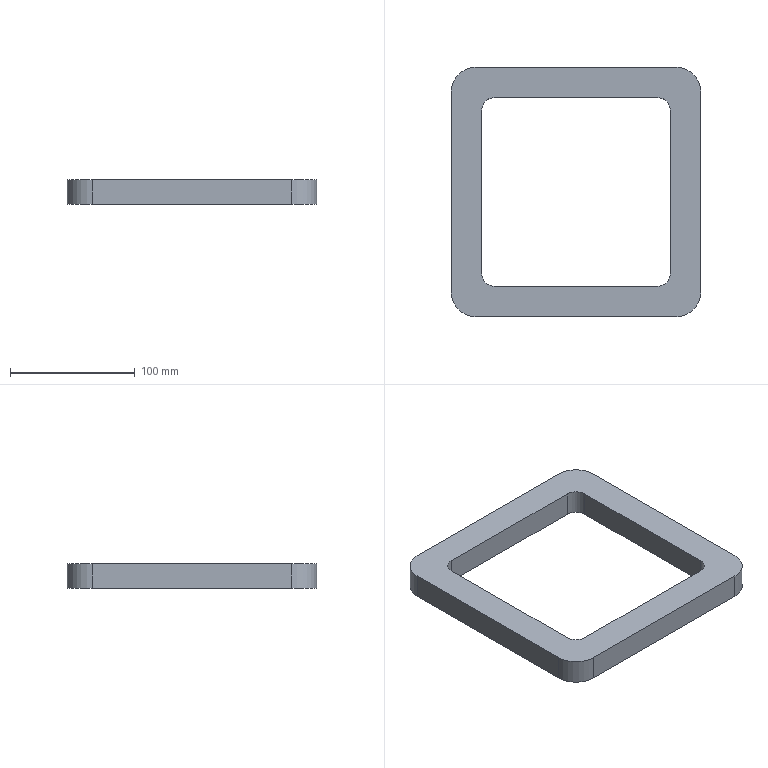Part | SolidWorks | features Fillet 2, Extrusion 1 | 1 solid | 18 faces | box 200 x 200 x 20 mm | volume 338830 mm3 | plane 10 | cylinder 8 | commonest cylinder face diameters 20 x4 40 x4
STEP:
#1=CARTESIAN_POINT('',(0.,180.,20.));
#2=VERTEX_POINT('',#1);
#3=CARTESIAN_POINT('',(0.,20.,20.));
#4=VERTEX_POINT('',#3);
#5=CARTESIAN_POINT('',(0.,0.,20.));
#6=DIRECTION('',(0.,-1.,0.));
#7=VECTOR('',#6,1000.);
#8=LINE('',#5,#7);
#9=EDGE_CURVE('',#2,#4,#8,.T.);
#10=ORIENTED_EDGE('',*,*,#9,.T.);
#11=CARTESIAN_POINT('',(20.,0.,20.));
#12=VERTEX_POINT('',#11);
#13=CARTESIAN_POINT('',(20.,20.,20.));
#14=DIRECTION('',(0.,0.,1.));
#15=DIRECTION('',(-1.,0.,0.));
#16=AXIS2_PLACEMENT_3D('',#13,#14,#15);
#17=CIRCLE('',#16,20.);
#18=EDGE_CURVE('',#4,#12,#17,.T.);
#19=ORIENTED_EDGE('',*,*,#18,.T.);
#20=CARTESIAN_POINT('',(180.,0.,20.));
#21=VERTEX_POINT('',#20);
#22=CARTESIAN_POINT('',(0.,0.,20.));
#23=DIRECTION('',(1.,0.,0.));
#24=VECTOR('',#23,1000.);
#25=LINE('',#22,#24);
#26=EDGE_CURVE('',#12,#21,#25,.T.);
#27=ORIENTED_EDGE('',*,*,#26,.T.);
#28=CARTESIAN_POINT('',(200.,20.,20.));
#29=VERTEX_POINT('',#28);
#30=CARTESIAN_POINT('',(180.,20.,20.));
#31=DIRECTION('',(0.,0.,1.));
#32=DIRECTION('',(-1.,0.,0.));
#33=AXIS2_PLACEMENT_3D('',#30,#31,#32);
#34=CIRCLE('',#33,20.);
#35=EDGE_CURVE('',#21,#29,#34,.T.);
#36=ORIENTED_EDGE('',*,*,#35,.T.);
#37=CARTESIAN_POINT('',(200.,180.,20.));
#38=VERTEX_POINT('',#37);
#39=CARTESIAN_POINT('',(200.,0.,20.));
#40=DIRECTION('',(0.,1.,0.));
#41=VECTOR('',#40,1000.);
#42=LINE('',#39,#41);
#43=EDGE_CURVE('',#29,#38,#42,.T.);
#44=ORIENTED_EDGE('',*,*,#43,.T.);
#45=CARTESIAN_POINT('',(180.,200.,20.));
#46=VERTEX_POINT('',#45);
#47=CARTESIAN_POINT('',(180.,180.,20.));
#48=DIRECTION('',(0.,0.,1.));
#49=DIRECTION('',(-1.,0.,0.));
#50=AXIS2_PLACEMENT_3D('',#47,#48,#49);
#51=CIRCLE('',#50,20.);
#52=EDGE_CURVE('',#38,#46,#51,.T.);
#53=ORIENTED_EDGE('',*,*,#52,.T.);
#54=CARTESIAN_POINT('',(20.,200.,20.));
#55=VERTEX_POINT('',#54);
#56=CARTESIAN_POINT('',(0.,200.,20.));
#57=DIRECTION('',(-1.,0.,0.));
#58=VECTOR('',#57,1000.);
#59=LINE('',#56,#58);
#60=EDGE_CURVE('',#46,#55,#59,.T.);
#61=ORIENTED_EDGE('',*,*,#60,.T.);
#62=CARTESIAN_POINT('',(20.,180.,20.));
#63=DIRECTION('',(0.,0.,1.));
#64=DIRECTION('',(-1.,0.,0.));
#65=AXIS2_PLACEMENT_3D('',#62,#63,#64);
#66=CIRCLE('',#65,20.);
#67=EDGE_CURVE('',#55,#2,#66,.T.);
#68=ORIENTED_EDGE('',*,*,#67,.T.);
#69=EDGE_LOOP('',(#10,#19,#27,#36,#44,#53,#61,#68));
#70=FACE_OUTER_BOUND('',#69,.T.);
#71=CARTESIAN_POINT('',(24.5,165.5,20.));
#72=VERTEX_POINT('',#71);
#73=CARTESIAN_POINT('',(24.5,34.5,20.));
#74=VERTEX_POINT('',#73);
#75=CARTESIAN_POINT('',(24.5,175.5,20.));
#76=DIRECTION('',(0.,-1.,0.));
#77=VECTOR('',#76,1000.);
#78=LINE('',#75,#77);
#79=EDGE_CURVE('',#72,#74,#78,.T.);
#80=ORIENTED_EDGE('',*,*,#79,.F.);
#81=CARTESIAN_POINT('',(34.5,175.5,20.));
#82=VERTEX_POINT('',#81);
#83=CARTESIAN_POINT('',(34.5,165.5,20.));
#84=DIRECTION('',(0.,0.,-1.));
#85=DIRECTION('',(-1.,0.,0.));
#86=AXIS2_PLACEMENT_3D('',#83,#84,#85);
#87=CIRCLE('',#86,10.);
#88=EDGE_CURVE('',#72,#82,#87,.T.);
#89=ORIENTED_EDGE('',*,*,#88,.T.);
#90=CARTESIAN_POINT('',(165.5,175.5,20.));
#91=VERTEX_POINT('',#90);
#92=CARTESIAN_POINT('',(24.5,175.5,20.));
#93=DIRECTION('',(-1.,0.,0.));
#94=VECTOR('',#93,1000.);
#95=LINE('',#92,#94);
#96=EDGE_CURVE('',#91,#82,#95,.T.);
#97=ORIENTED_EDGE('',*,*,#96,.F.);
#98=CARTESIAN_POINT('',(175.5,165.5,20.));
#99=VERTEX_POINT('',#98);
#100=CARTESIAN_POINT('',(165.5,165.5,20.));
#101=DIRECTION('',(0.,0.,-1.));
#102=DIRECTION('',(-1.,0.,0.));
#103=AXIS2_PLACEMENT_3D('',#100,#101,#102);
#104=CIRCLE('',#103,10.);
#105=EDGE_CURVE('',#91,#99,#104,.T.);
#106=ORIENTED_EDGE('',*,*,#105,.T.);
#107=CARTESIAN_POINT('',(175.5,34.5,20.));
#108=VERTEX_POINT('',#107);
#109=CARTESIAN_POINT('',(175.5,175.5,20.));
#110=DIRECTION('',(0.,1.,0.));
#111=VECTOR('',#110,1000.);
#112=LINE('',#109,#111);
#113=EDGE_CURVE('',#108,#99,#112,.T.);
#114=ORIENTED_EDGE('',*,*,#113,.F.);
#115=CARTESIAN_POINT('',(165.5,24.5,20.));
#116=VERTEX_POINT('',#115);
#117=CARTESIAN_POINT('',(165.5,34.5,20.));
#118=DIRECTION('',(0.,0.,-1.));
#119=DIRECTION('',(-1.,0.,0.));
#120=AXIS2_PLACEMENT_3D('',#117,#118,#119);
#121=CIRCLE('',#120,10.);
#122=EDGE_CURVE('',#108,#116,#121,.T.);
#123=ORIENTED_EDGE('',*,*,#122,.T.);
#124=CARTESIAN_POINT('',(34.5,24.5,20.));
#125=VERTEX_POINT('',#124);
#126=CARTESIAN_POINT('',(24.5,24.5,20.));
#127=DIRECTION('',(1.,0.,0.));
#128=VECTOR('',#127,1000.);
#129=LINE('',#126,#128);
#130=EDGE_CURVE('',#125,#116,#129,.T.);
#131=ORIENTED_EDGE('',*,*,#130,.F.);
#132=CARTESIAN_POINT('',(34.5,34.5,20.));
#133=DIRECTION('',(0.,0.,-1.));
#134=DIRECTION('',(-1.,0.,0.));
#135=AXIS2_PLACEMENT_3D('',#132,#133,#134);
#136=CIRCLE('',#135,10.);
#137=EDGE_CURVE('',#125,#74,#136,.T.);
#138=ORIENTED_EDGE('',*,*,#137,.T.);
#139=EDGE_LOOP('',(#80,#89,#97,#106,#114,#123,#131,#138));
#140=FACE_BOUND('',#139,.T.);
#141=CARTESIAN_POINT('',(0.,0.,20.));
#142=DIRECTION('',(0.,0.,-1.));
#143=DIRECTION('',(-1.,0.,0.));
#144=AXIS2_PLACEMENT_3D('',#141,#142,#143);
#145=PLANE('',#144);
#146=ADVANCED_FACE('',(#70,#140),#145,.F.);
#147=CARTESIAN_POINT('',(20.,0.,0.));
#148=VERTEX_POINT('',#147);
#149=CARTESIAN_POINT('',(180.,0.,0.));
#150=VERTEX_POINT('',#149);
#151=CARTESIAN_POINT('',(0.,0.,0.));
#152=DIRECTION('',(1.,0.,0.));
#153=VECTOR('',#152,1000.);
#154=LINE('',#151,#153);
#155=EDGE_CURVE('',#148,#150,#154,.T.);
#156=ORIENTED_EDGE('',*,*,#155,.F.);
#157=CARTESIAN_POINT('',(0.,20.,0.));
#158=VERTEX_POINT('',#157);
#159=CARTESIAN_POINT('',(20.,20.,0.));
#160=DIRECTION('',(0.,0.,-1.));
#161=DIRECTION('',(-1.,0.,0.));
#162=AXIS2_PLACEMENT_3D('',#159,#160,#161);
#163=CIRCLE('',#162,20.);
#164=EDGE_CURVE('',#148,#158,#163,.T.);
#165=ORIENTED_EDGE('',*,*,#164,.T.);
#166=CARTESIAN_POINT('',(0.,180.,0.));
#167=VERTEX_POINT('',#166);
#168=CARTESIAN_POINT('',(0.,0.,0.));
#169=DIRECTION('',(0.,-1.,0.));
#170=VECTOR('',#169,1000.);
#171=LINE('',#168,#170);
#172=EDGE_CURVE('',#167,#158,#171,.T.);
#173=ORIENTED_EDGE('',*,*,#172,.F.);
#174=CARTESIAN_POINT('',(20.,200.,0.));
#175=VERTEX_POINT('',#174);
#176=CARTESIAN_POINT('',(20.,180.,0.));
#177=DIRECTION('',(0.,0.,-1.));
#178=DIRECTION('',(-1.,0.,0.));
#179=AXIS2_PLACEMENT_3D('',#176,#177,#178);
#180=CIRCLE('',#179,20.);
#181=EDGE_CURVE('',#167,#175,#180,.T.);
#182=ORIENTED_EDGE('',*,*,#181,.T.);
#183=CARTESIAN_POINT('',(180.,200.,0.));
#184=VERTEX_POINT('',#183);
#185=CARTESIAN_POINT('',(0.,200.,0.));
#186=DIRECTION('',(-1.,0.,0.));
#187=VECTOR('',#186,1000.);
#188=LINE('',#185,#187);
#189=EDGE_CURVE('',#184,#175,#188,.T.);
#190=ORIENTED_EDGE('',*,*,#189,.F.);
#191=CARTESIAN_POINT('',(200.,180.,0.));
#192=VERTEX_POINT('',#191);
#193=CARTESIAN_POINT('',(180.,180.,0.));
#194=DIRECTION('',(0.,0.,-1.));
#195=DIRECTION('',(-1.,0.,0.));
#196=AXIS2_PLACEMENT_3D('',#193,#194,#195);
#197=CIRCLE('',#196,20.);
#198=EDGE_CURVE('',#184,#192,#197,.T.);
#199=ORIENTED_EDGE('',*,*,#198,.T.);
#200=CARTESIAN_POINT('',(200.,20.,0.));
#201=VERTEX_POINT('',#200);
#202=CARTESIAN_POINT('',(200.,0.,0.));
#203=DIRECTION('',(0.,1.,0.));
#204=VECTOR('',#203,1000.);
#205=LINE('',#202,#204);
#206=EDGE_CURVE('',#201,#192,#205,.T.);
#207=ORIENTED_EDGE('',*,*,#206,.F.);
#208=CARTESIAN_POINT('',(180.,20.,0.));
#209=DIRECTION('',(0.,0.,-1.));
#210=DIRECTION('',(-1.,0.,0.));
#211=AXIS2_PLACEMENT_3D('',#208,#209,#210);
#212=CIRCLE('',#211,20.);
#213=EDGE_CURVE('',#201,#150,#212,.T.);
#214=ORIENTED_EDGE('',*,*,#213,.T.);
#215=EDGE_LOOP('',(#156,#165,#173,#182,#190,#199,#207,#214));
#216=FACE_OUTER_BOUND('',#215,.T.);
#217=CARTESIAN_POINT('',(175.5,34.5,0.));
#218=VERTEX_POINT('',#217);
#219=CARTESIAN_POINT('',(175.5,165.5,0.));
#220=VERTEX_POINT('',#219);
#221=CARTESIAN_POINT('',(175.5,175.5,0.));
#222=DIRECTION('',(0.,1.,0.));
#223=VECTOR('',#222,1000.);
#224=LINE('',#221,#223);
#225=EDGE_CURVE('',#218,#220,#224,.T.);
#226=ORIENTED_EDGE('',*,*,#225,.T.);
#227=CARTESIAN_POINT('',(165.5,175.5,0.));
#228=VERTEX_POINT('',#227);
#229=CARTESIAN_POINT('',(165.5,165.5,0.));
#230=DIRECTION('',(0.,0.,1.));
#231=DIRECTION('',(-1.,0.,0.));
#232=AXIS2_PLACEMENT_3D('',#229,#230,#231);
#233=CIRCLE('',#232,10.);
#234=EDGE_CURVE('',#220,#228,#233,.T.);
#235=ORIENTED_EDGE('',*,*,#234,.T.);
#236=CARTESIAN_POINT('',(34.5,175.5,0.));
#237=VERTEX_POINT('',#236);
#238=CARTESIAN_POINT('',(24.5,175.5,0.));
#239=DIRECTION('',(-1.,0.,0.));
#240=VECTOR('',#239,1000.);
#241=LINE('',#238,#240);
#242=EDGE_CURVE('',#228,#237,#241,.T.);
#243=ORIENTED_EDGE('',*,*,#242,.T.);
#244=CARTESIAN_POINT('',(24.5,165.5,0.));
#245=VERTEX_POINT('',#244);
#246=CARTESIAN_POINT('',(34.5,165.5,0.));
#247=DIRECTION('',(0.,0.,1.));
#248=DIRECTION('',(-1.,0.,0.));
#249=AXIS2_PLACEMENT_3D('',#246,#247,#248);
#250=CIRCLE('',#249,10.);
#251=EDGE_CURVE('',#237,#245,#250,.T.);
#252=ORIENTED_EDGE('',*,*,#251,.T.);
#253=CARTESIAN_POINT('',(24.5,34.5,0.));
#254=VERTEX_POINT('',#253);
#255=CARTESIAN_POINT('',(24.5,175.5,0.));
#256=DIRECTION('',(0.,-1.,0.));
#257=VECTOR('',#256,1000.);
#258=LINE('',#255,#257);
#259=EDGE_CURVE('',#245,#254,#258,.T.);
#260=ORIENTED_EDGE('',*,*,#259,.T.);
#261=CARTESIAN_POINT('',(34.5,24.5,0.));
#262=VERTEX_POINT('',#261);
#263=CARTESIAN_POINT('',(34.5,34.5,0.));
#264=DIRECTION('',(0.,0.,1.));
#265=DIRECTION('',(-1.,0.,0.));
#266=AXIS2_PLACEMENT_3D('',#263,#264,#265);
#267=CIRCLE('',#266,10.);
#268=EDGE_CURVE('',#254,#262,#267,.T.);
#269=ORIENTED_EDGE('',*,*,#268,.T.);
#270=CARTESIAN_POINT('',(165.5,24.5,0.));
#271=VERTEX_POINT('',#270);
#272=CARTESIAN_POINT('',(24.5,24.5,0.));
#273=DIRECTION('',(1.,0.,0.));
#274=VECTOR('',#273,1000.);
#275=LINE('',#272,#274);
#276=EDGE_CURVE('',#262,#271,#275,.T.);
#277=ORIENTED_EDGE('',*,*,#276,.T.);
#278=CARTESIAN_POINT('',(165.5,34.5,0.));
#279=DIRECTION('',(0.,0.,1.));
#280=DIRECTION('',(-1.,0.,0.));
#281=AXIS2_PLACEMENT_3D('',#278,#279,#280);
#282=CIRCLE('',#281,10.);
#283=EDGE_CURVE('',#271,#218,#282,.T.);
#284=ORIENTED_EDGE('',*,*,#283,.T.);
#285=EDGE_LOOP('',(#226,#235,#243,#252,#260,#269,#277,#284));
#286=FACE_BOUND('',#285,.T.);
#287=CARTESIAN_POINT('',(0.,0.,0.));
#288=DIRECTION('',(0.,0.,-1.));
#289=DIRECTION('',(-1.,0.,0.));
#290=AXIS2_PLACEMENT_3D('',#287,#288,#289);
#291=PLANE('',#290);
#292=ADVANCED_FACE('',(#216,#286),#291,.T.);
#293=ORIENTED_EDGE('',*,*,#172,.T.);
#294=CARTESIAN_POINT('',(0.,20.,20.));
#295=DIRECTION('',(0.,0.,1.));
#296=VECTOR('',#295,1000.);
#297=LINE('',#294,#296);
#298=EDGE_CURVE('',#158,#4,#297,.T.);
#299=ORIENTED_EDGE('',*,*,#298,.T.);
#300=ORIENTED_EDGE('',*,*,#9,.F.);
#301=CARTESIAN_POINT('',(0.,180.,20.));
#302=DIRECTION('',(0.,0.,-1.));
#303=VECTOR('',#302,1000.);
#304=LINE('',#301,#303);
#305=EDGE_CURVE('',#2,#167,#304,.T.);
#306=ORIENTED_EDGE('',*,*,#305,.T.);
#307=EDGE_LOOP('',(#293,#299,#300,#306));
#308=FACE_OUTER_BOUND('',#307,.T.);
#309=CARTESIAN_POINT('',(0.,0.,20.));
#310=DIRECTION('',(1.,0.,0.));
#311=DIRECTION('',(0.,0.,-1.));
#312=AXIS2_PLACEMENT_3D('',#309,#310,#311);
#313=PLANE('',#312);
#314=ADVANCED_FACE('',(#308),#313,.F.);
#315=ORIENTED_EDGE('',*,*,#26,.F.);
#316=CARTESIAN_POINT('',(20.,0.,20.));
#317=DIRECTION('',(0.,0.,-1.));
#318=VECTOR('',#317,1000.);
#319=LINE('',#316,#318);
#320=EDGE_CURVE('',#12,#148,#319,.T.);
#321=ORIENTED_EDGE('',*,*,#320,.T.);
#322=ORIENTED_EDGE('',*,*,#155,.T.);
#323=CARTESIAN_POINT('',(180.,0.,20.));
#324=DIRECTION('',(0.,0.,1.));
#325=VECTOR('',#324,1000.);
#326=LINE('',#323,#325);
#327=EDGE_CURVE('',#150,#21,#326,.T.);
#328=ORIENTED_EDGE('',*,*,#327,.T.);
#329=EDGE_LOOP('',(#315,#321,#322,#328));
#330=FACE_OUTER_BOUND('',#329,.T.);
#331=CARTESIAN_POINT('',(0.,0.,20.));
#332=DIRECTION('',(0.,1.,0.));
#333=DIRECTION('',(0.,0.,1.));
#334=AXIS2_PLACEMENT_3D('',#331,#332,#333);
#335=PLANE('',#334);
#336=ADVANCED_FACE('',(#330),#335,.F.);
#337=ORIENTED_EDGE('',*,*,#43,.F.);
#338=CARTESIAN_POINT('',(200.,20.,20.));
#339=DIRECTION('',(0.,0.,-1.));
#340=VECTOR('',#339,1000.);
#341=LINE('',#338,#340);
#342=EDGE_CURVE('',#29,#201,#341,.T.);
#343=ORIENTED_EDGE('',*,*,#342,.T.);
#344=ORIENTED_EDGE('',*,*,#206,.T.);
#345=CARTESIAN_POINT('',(200.,180.,20.));
#346=DIRECTION('',(0.,0.,1.));
#347=VECTOR('',#346,1000.);
#348=LINE('',#345,#347);
#349=EDGE_CURVE('',#192,#38,#348,.T.);
#350=ORIENTED_EDGE('',*,*,#349,.T.);
#351=EDGE_LOOP('',(#337,#343,#344,#350));
#352=FACE_OUTER_BOUND('',#351,.T.);
#353=CARTESIAN_POINT('',(200.,0.,20.));
#354=DIRECTION('',(-1.,0.,0.));
#355=DIRECTION('',(0.,0.,1.));
#356=AXIS2_PLACEMENT_3D('',#353,#354,#355);
#357=PLANE('',#356);
#358=ADVANCED_FACE('',(#352),#357,.F.);
#359=ORIENTED_EDGE('',*,*,#60,.F.);
#360=CARTESIAN_POINT('',(180.,200.,20.));
#361=DIRECTION('',(0.,0.,-1.));
#362=VECTOR('',#361,1000.);
#363=LINE('',#360,#362);
#364=EDGE_CURVE('',#46,#184,#363,.T.);
#365=ORIENTED_EDGE('',*,*,#364,.T.);
#366=ORIENTED_EDGE('',*,*,#189,.T.);
#367=CARTESIAN_POINT('',(20.,200.,20.));
#368=DIRECTION('',(0.,0.,1.));
#369=VECTOR('',#368,1000.);
#370=LINE('',#367,#369);
#371=EDGE_CURVE('',#175,#55,#370,.T.);
#372=ORIENTED_EDGE('',*,*,#371,.T.);
#373=EDGE_LOOP('',(#359,#365,#366,#372));
#374=FACE_OUTER_BOUND('',#373,.T.);
#375=CARTESIAN_POINT('',(0.,200.,20.));
#376=DIRECTION('',(0.,-1.,0.));
#377=DIRECTION('',(0.,0.,-1.));
#378=AXIS2_PLACEMENT_3D('',#375,#376,#377);
#379=PLANE('',#378);
#380=ADVANCED_FACE('',(#374),#379,.F.);
#381=ORIENTED_EDGE('',*,*,#259,.F.);
#382=CARTESIAN_POINT('',(24.5,165.5,20.));
#383=DIRECTION('',(0.,0.,1.));
#384=VECTOR('',#383,1000.);
#385=LINE('',#382,#384);
#386=EDGE_CURVE('',#245,#72,#385,.T.);
#387=ORIENTED_EDGE('',*,*,#386,.T.);
#388=ORIENTED_EDGE('',*,*,#79,.T.);
#389=CARTESIAN_POINT('',(24.5,34.5,0.));
#390=DIRECTION('',(0.,0.,-1.));
#391=VECTOR('',#390,1000.);
#392=LINE('',#389,#391);
#393=EDGE_CURVE('',#74,#254,#392,.T.);
#394=ORIENTED_EDGE('',*,*,#393,.T.);
#395=EDGE_LOOP('',(#381,#387,#388,#394));
#396=FACE_OUTER_BOUND('',#395,.T.);
#397=CARTESIAN_POINT('',(24.5,175.5,20.));
#398=DIRECTION('',(1.,0.,0.));
#399=DIRECTION('',(0.,1.,0.));
#400=AXIS2_PLACEMENT_3D('',#397,#398,#399);
#401=PLANE('',#400);
#402=ADVANCED_FACE('',(#396),#401,.T.);
#403=ORIENTED_EDGE('',*,*,#130,.T.);
#404=CARTESIAN_POINT('',(165.5,24.5,0.));
#405=DIRECTION('',(0.,0.,-1.));
#406=VECTOR('',#405,1000.);
#407=LINE('',#404,#406);
#408=EDGE_CURVE('',#116,#271,#407,.T.);
#409=ORIENTED_EDGE('',*,*,#408,.T.);
#410=ORIENTED_EDGE('',*,*,#276,.F.);
#411=CARTESIAN_POINT('',(34.5,24.5,20.));
#412=DIRECTION('',(0.,0.,1.));
#413=VECTOR('',#412,1000.);
#414=LINE('',#411,#413);
#415=EDGE_CURVE('',#262,#125,#414,.T.);
#416=ORIENTED_EDGE('',*,*,#415,.T.);
#417=EDGE_LOOP('',(#403,#409,#410,#416));
#418=FACE_OUTER_BOUND('',#417,.T.);
#419=CARTESIAN_POINT('',(24.5,24.5,20.));
#420=DIRECTION('',(0.,1.,0.));
#421=DIRECTION('',(0.,0.,1.));
#422=AXIS2_PLACEMENT_3D('',#419,#420,#421);
#423=PLANE('',#422);
#424=ADVANCED_FACE('',(#418),#423,.T.);
#425=ORIENTED_EDGE('',*,*,#225,.F.);
#426=CARTESIAN_POINT('',(175.5,34.5,20.));
#427=DIRECTION('',(0.,0.,1.));
#428=VECTOR('',#427,1000.);
#429=LINE('',#426,#428);
#430=EDGE_CURVE('',#218,#108,#429,.T.);
#431=ORIENTED_EDGE('',*,*,#430,.T.);
#432=ORIENTED_EDGE('',*,*,#113,.T.);
#433=CARTESIAN_POINT('',(175.5,165.5,0.));
#434=DIRECTION('',(0.,0.,-1.));
#435=VECTOR('',#434,1000.);
#436=LINE('',#433,#435);
#437=EDGE_CURVE('',#99,#220,#436,.T.);
#438=ORIENTED_EDGE('',*,*,#437,.T.);
#439=EDGE_LOOP('',(#425,#431,#432,#438));
#440=FACE_OUTER_BOUND('',#439,.T.);
#441=CARTESIAN_POINT('',(175.5,175.5,20.));
#442=DIRECTION('',(-1.,0.,0.));
#443=DIRECTION('',(0.,-1.,0.));
#444=AXIS2_PLACEMENT_3D('',#441,#442,#443);
#445=PLANE('',#444);
#446=ADVANCED_FACE('',(#440),#445,.T.);
#447=ORIENTED_EDGE('',*,*,#242,.F.);
#448=CARTESIAN_POINT('',(165.5,175.5,20.));
#449=DIRECTION('',(0.,0.,1.));
#450=VECTOR('',#449,1000.);
#451=LINE('',#448,#450);
#452=EDGE_CURVE('',#228,#91,#451,.T.);
#453=ORIENTED_EDGE('',*,*,#452,.T.);
#454=ORIENTED_EDGE('',*,*,#96,.T.);
#455=CARTESIAN_POINT('',(34.5,175.5,0.));
#456=DIRECTION('',(0.,0.,-1.));
#457=VECTOR('',#456,1000.);
#458=LINE('',#455,#457);
#459=EDGE_CURVE('',#82,#237,#458,.T.);
#460=ORIENTED_EDGE('',*,*,#459,.T.);
#461=EDGE_LOOP('',(#447,#453,#454,#460));
#462=FACE_OUTER_BOUND('',#461,.T.);
#463=CARTESIAN_POINT('',(24.5,175.5,20.));
#464=DIRECTION('',(0.,-1.,0.));
#465=DIRECTION('',(0.,0.,-1.));
#466=AXIS2_PLACEMENT_3D('',#463,#464,#465);
#467=PLANE('',#466);
#468=ADVANCED_FACE('',(#462),#467,.T.);
#469=ORIENTED_EDGE('',*,*,#18,.F.);
#470=ORIENTED_EDGE('',*,*,#298,.F.);
#471=ORIENTED_EDGE('',*,*,#164,.F.);
#472=ORIENTED_EDGE('',*,*,#320,.F.);
#473=EDGE_LOOP('',(#469,#470,#471,#472));
#474=FACE_OUTER_BOUND('',#473,.T.);
#475=CARTESIAN_POINT('',(20.,20.,20.));
#476=DIRECTION('',(0.,0.,-1.));
#477=DIRECTION('',(-1.,0.,0.));
#478=AXIS2_PLACEMENT_3D('',#475,#476,#477);
#479=CYLINDRICAL_SURFACE('',#478,20.);
#480=ADVANCED_FACE('',(#474),#479,.T.);
#481=ORIENTED_EDGE('',*,*,#35,.F.);
#482=ORIENTED_EDGE('',*,*,#327,.F.);
#483=ORIENTED_EDGE('',*,*,#213,.F.);
#484=ORIENTED_EDGE('',*,*,#342,.F.);
#485=EDGE_LOOP('',(#481,#482,#483,#484));
#486=FACE_OUTER_BOUND('',#485,.T.);
#487=CARTESIAN_POINT('',(180.,20.,20.));
#488=DIRECTION('',(0.,0.,-1.));
#489=DIRECTION('',(-1.,0.,0.));
#490=AXIS2_PLACEMENT_3D('',#487,#488,#489);
#491=CYLINDRICAL_SURFACE('',#490,20.);
#492=ADVANCED_FACE('',(#486),#491,.T.);
#493=ORIENTED_EDGE('',*,*,#52,.F.);
#494=ORIENTED_EDGE('',*,*,#349,.F.);
#495=ORIENTED_EDGE('',*,*,#198,.F.);
#496=ORIENTED_EDGE('',*,*,#364,.F.);
#497=EDGE_LOOP('',(#493,#494,#495,#496));
#498=FACE_OUTER_BOUND('',#497,.T.);
#499=CARTESIAN_POINT('',(180.,180.,20.));
#500=DIRECTION('',(0.,0.,-1.));
#501=DIRECTION('',(-1.,0.,0.));
#502=AXIS2_PLACEMENT_3D('',#499,#500,#501);
#503=CYLINDRICAL_SURFACE('',#502,20.);
#504=ADVANCED_FACE('',(#498),#503,.T.);
#505=ORIENTED_EDGE('',*,*,#67,.F.);
#506=ORIENTED_EDGE('',*,*,#371,.F.);
#507=ORIENTED_EDGE('',*,*,#181,.F.);
#508=ORIENTED_EDGE('',*,*,#305,.F.);
#509=EDGE_LOOP('',(#505,#506,#507,#508));
#510=FACE_OUTER_BOUND('',#509,.T.);
#511=CARTESIAN_POINT('',(20.,180.,20.));
#512=DIRECTION('',(0.,0.,-1.));
#513=DIRECTION('',(-1.,0.,0.));
#514=AXIS2_PLACEMENT_3D('',#511,#512,#513);
#515=CYLINDRICAL_SURFACE('',#514,20.);
#516=ADVANCED_FACE('',(#510),#515,.T.);
#517=ORIENTED_EDGE('',*,*,#122,.F.);
#518=ORIENTED_EDGE('',*,*,#430,.F.);
#519=ORIENTED_EDGE('',*,*,#283,.F.);
#520=ORIENTED_EDGE('',*,*,#408,.F.);
#521=EDGE_LOOP('',(#517,#518,#519,#520));
#522=FACE_OUTER_BOUND('',#521,.T.);
#523=CARTESIAN_POINT('',(165.5,34.5,20.));
#524=DIRECTION('',(0.,0.,1.));
#525=DIRECTION('',(1.,0.,0.));
#526=AXIS2_PLACEMENT_3D('',#523,#524,#525);
#527=CYLINDRICAL_SURFACE('',#526,10.);
#528=ADVANCED_FACE('',(#522),#527,.F.);
#529=ORIENTED_EDGE('',*,*,#105,.F.);
#530=ORIENTED_EDGE('',*,*,#452,.F.);
#531=ORIENTED_EDGE('',*,*,#234,.F.);
#532=ORIENTED_EDGE('',*,*,#437,.F.);
#533=EDGE_LOOP('',(#529,#530,#531,#532));
#534=FACE_OUTER_BOUND('',#533,.T.);
#535=CARTESIAN_POINT('',(165.5,165.5,20.));
#536=DIRECTION('',(0.,0.,1.));
#537=DIRECTION('',(1.,0.,0.));
#538=AXIS2_PLACEMENT_3D('',#535,#536,#537);
#539=CYLINDRICAL_SURFACE('',#538,10.);
#540=ADVANCED_FACE('',(#534),#539,.F.);
#541=ORIENTED_EDGE('',*,*,#88,.F.);
#542=ORIENTED_EDGE('',*,*,#386,.F.);
#543=ORIENTED_EDGE('',*,*,#251,.F.);
#544=ORIENTED_EDGE('',*,*,#459,.F.);
#545=EDGE_LOOP('',(#541,#542,#543,#544));
#546=FACE_OUTER_BOUND('',#545,.T.);
#547=CARTESIAN_POINT('',(34.5,165.5,20.));
#548=DIRECTION('',(0.,0.,1.));
#549=DIRECTION('',(1.,0.,0.));
#550=AXIS2_PLACEMENT_3D('',#547,#548,#549);
#551=CYLINDRICAL_SURFACE('',#550,10.);
#552=ADVANCED_FACE('',(#546),#551,.F.);
#553=ORIENTED_EDGE('',*,*,#137,.F.);
#554=ORIENTED_EDGE('',*,*,#415,.F.);
#555=ORIENTED_EDGE('',*,*,#268,.F.);
#556=ORIENTED_EDGE('',*,*,#393,.F.);
#557=EDGE_LOOP('',(#553,#554,#555,#556));
#558=FACE_OUTER_BOUND('',#557,.T.);
#559=CARTESIAN_POINT('',(34.5,34.5,20.));
#560=DIRECTION('',(0.,0.,1.));
#561=DIRECTION('',(1.,0.,0.));
#562=AXIS2_PLACEMENT_3D('',#559,#560,#561);
#563=CYLINDRICAL_SURFACE('',#562,10.);
#564=ADVANCED_FACE('',(#558),#563,.F.);
#565=CLOSED_SHELL('',(#146,#292,#314,#336,#358,#380,#402,#424,#446,#468,#480,#492,#504,#516,#528,#540,#552,#564));
#566=MANIFOLD_SOLID_BREP('',#565);
#567=CARTESIAN_POINT('',(0.,0.,0.));
#568=DIRECTION('',(0.,0.,1.));
#569=DIRECTION('',(1.,0.,0.));
#570=AXIS2_PLACEMENT_3D('',#567,#568,#569);
#571=(LENGTH_UNIT()NAMED_UNIT(*)SI_UNIT(.MILLI.,.METRE.));
#572=UNCERTAINTY_MEASURE_WITH_UNIT(LENGTH_MEASURE(0.00001),#571,'','');
#573=(NAMED_UNIT(*)PLANE_ANGLE_UNIT()SI_UNIT($,.RADIAN.));
#574=(NAMED_UNIT(*)SI_UNIT($,.STERADIAN.)SOLID_ANGLE_UNIT());
#575=(GEOMETRIC_REPRESENTATION_CONTEXT(3)GLOBAL_UNCERTAINTY_ASSIGNED_CONTEXT((#572))GLOBAL_UNIT_ASSIGNED_CONTEXT((#571,#573,#574))REPRESENTATION_CONTEXT('',''));
#576=ADVANCED_BREP_SHAPE_REPRESENTATION('',(#566,#570),#575);